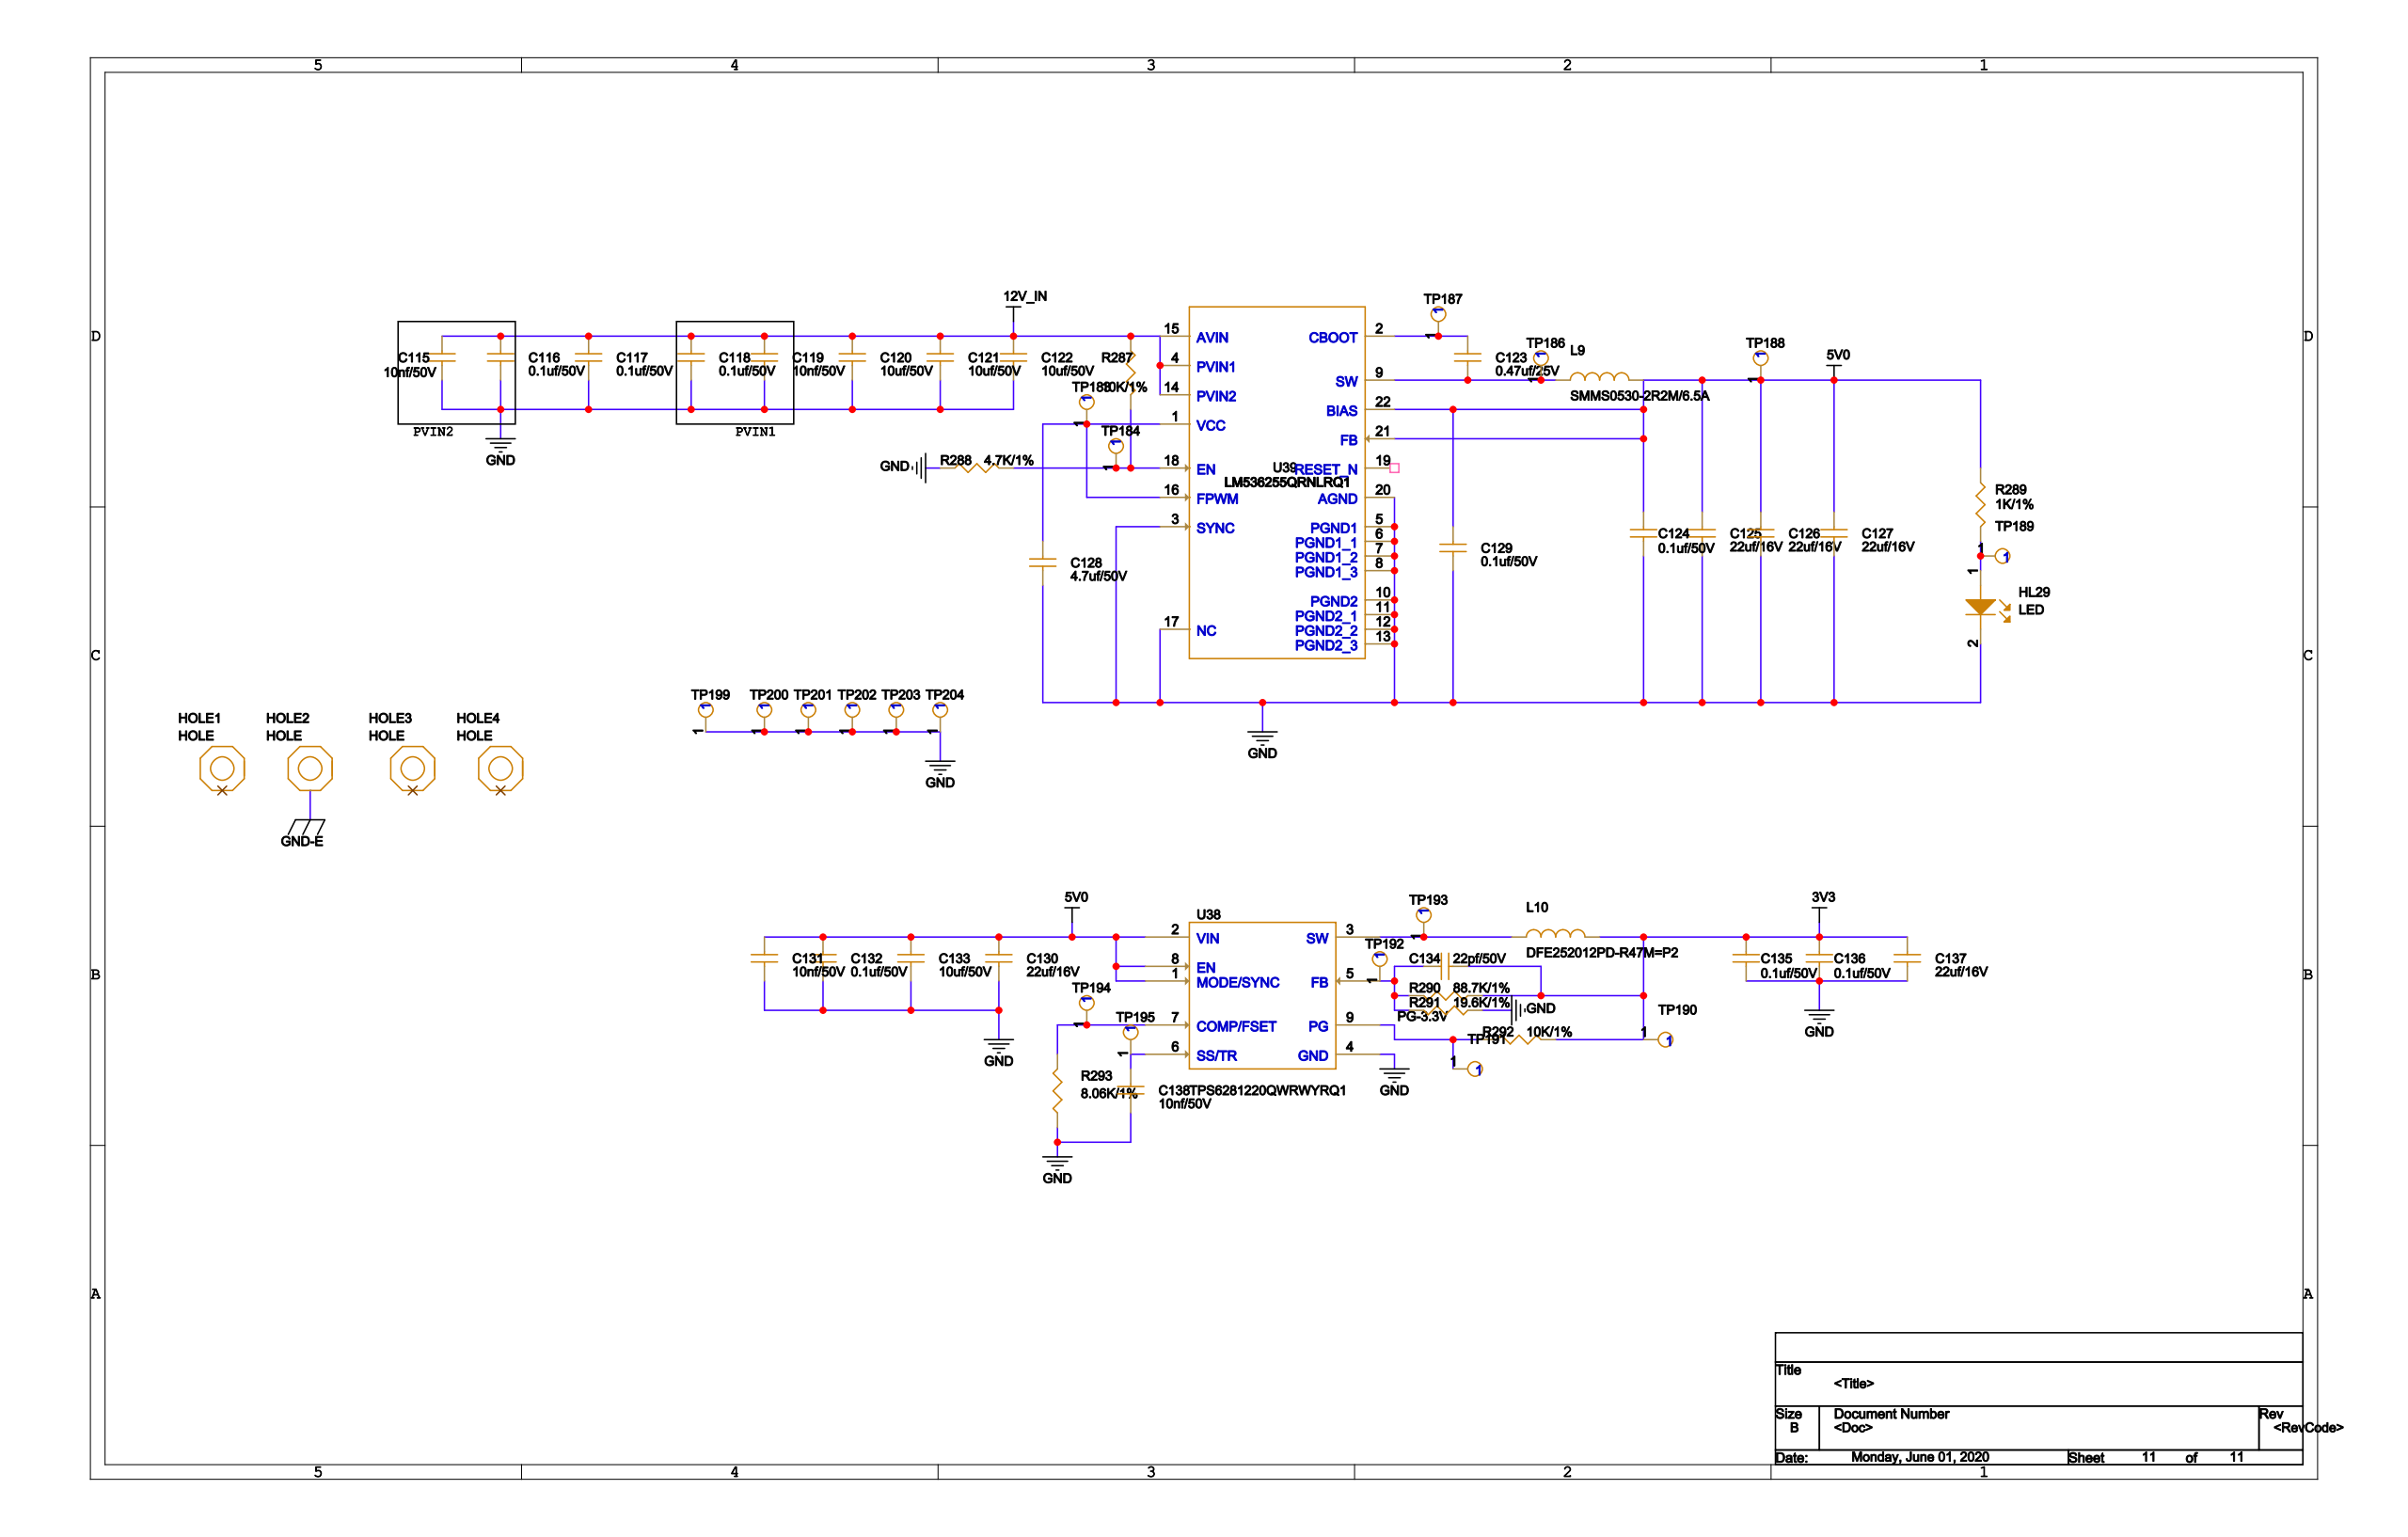Circuit board | Cadence Allegro | 792 parts | 400 nets | one sheet of the schematic
Parts on this sheet (reference | value | footprint):
C115 | 10nf/50V | C0402
C116 | 0.1uf/50V | C0402
C117 | 0.1uf/50V | C0402
C118 | 0.1uf/50V | C0402
C119 | 10nf/50V | C0402
C120 | 10uf/50V | C0805
C121 | 10uf/50V | C0805
C122 | 10uf/50V | C0805
C123 | 0.47uf/25V | C0402
C124 | 0.1uf/50V | C0402
C125 | 22uf/16V | C1210
C126 | 22uf/16V | C1210
C127 | 22uf/16V | C1210
C128 | 4.7uf/50V | C0805
C129 | 0.1uf/50V | C0402
C130 | 22uf/16V | C1210
C131 | 10nf/50V | C0402
C132 | 0.1uf/50V | C0402
C133 | 10uf/50V | C0805
C134 | 22pf/50V | C0402
C135 | 0.1uf/50V | C0402
C136 | 0.1uf/50V | C0402
C137 | 22uf/16V | C1210
C138 | 10nf/50V | C0402
HL29 | LED | LED0603
HOLE2 | HOLE | HOLEPAD_80X35
L9 | SMMS0530-2R2M/6.5A | SM_IND_5L
L10 | DFE252012PD-R47M=P2 | SM_IND_3L
R287 | 10K/1% | 0402
R288 | 4.7K/1% | 0402
R289 | 1K/1% | R0603
R290 | 88.7K/1% | 0603
R291 | 19.6K/1% | 0603
R292 | 10K/1% | 0603
R293 | 8.06K/1% | 0402
TP183 | TESTPOINT | TESTPOINT-33MIL
TP184 | TESTPOINT | TESTPOINT-33MIL
TP186 | TESTPOINT | TESTPOINT-33MIL
TP187 | TESTPOINT | TESTPOINT-33MIL
TP188 | TESTPOINT | TESTPOINT-33MIL
TP189 | TESTPOINT | TESTPOINT-33MIL
TP190 | TESTPOINT | TESTPOINT-33MIL
TP191 | TESTPOINT | TESTPOINT-33MIL
TP192 | TESTPOINT | TESTPOINT-33MIL
TP193 | TESTPOINT | TESTPOINT-33MIL
TP194 | TESTPOINT | TESTPOINT-33MIL
TP195 | TESTPOINT | TESTPOINT-33MIL
TP199 | TESTPOINT | TESTPOINT-33MIL
TP200 | TESTPOINT | TESTPOINT-33MIL
TP201 | TESTPOINT | TESTPOINT-33MIL
TP202 | TESTPOINT | TESTPOINT-33MIL
TP203 | TESTPOINT | TESTPOINT-33MIL
TP204 | TESTPOINT | TESTPOINT-33MIL
U38 | TPS6281220QWRWYRQ1 | RWY0009A
U39 | LM536255QRNLRQ1 | RNL0022A_NV
Nets of these parts (net: part-pin ...):
3V3: C134-2 C135-1 C136-1 C137-1 L10-2 R290-1 R292-2 TP190-1
GND-E: HOLE2-1
GND: C115-2 C116-2 C117-2 C118-2 C119-2 C120-2 C121-2 C122-2 C124-2 C125-2 C126-2 C127-2 C128-2 C129-2 C130-2 C131-2 C132-2 C133-2 C135-2 C136-2 C137-2 C138-2 HL29-2 R288-1 R291-1 R293-1 TP199-1 TP200-1 TP201-1 TP202-1 TP203-1 TP204-1 U38-4 U39-3 U39-5 U39-6 U39-7 U39-8 U39-10 U39-11 U39-12 U39-13 U39-17 U39-20
5V0: C124-1 C125-1 C126-1 C127-1 C129-1 C130-1 C131-1 C132-1 C133-1 L9-2 R289-1 TP188-1 U38-1 U38-2 U38-8 U39-21 U39-22
12V_IN: C115-1 C116-1 C117-1 C118-1 C119-1 C120-1 C121-1 C122-1 R287-1 U39-4 U39-14 U39-15
N7539499: L10-1 TP193-1 U38-3
PG-3.3V: R292-1 TP191-1 U38-9
N7538390: R293-2 TP194-1 U38-7
N7278733: C128-1 TP183-1 U39-1 U39-16
N7278425: R287-2 R288-2 TP184-1 U39-18
N7278841: C123-2 L9-1 TP186-1 U39-9
N7278865: C123-1 TP187-1 U39-2
N7845429: HL29-1 R289-2 TP189-1
N7539563: C134-1 R290-2 R291-2 TP192-1 U38-5
N7538521: C138-1 TP195-1 U38-6